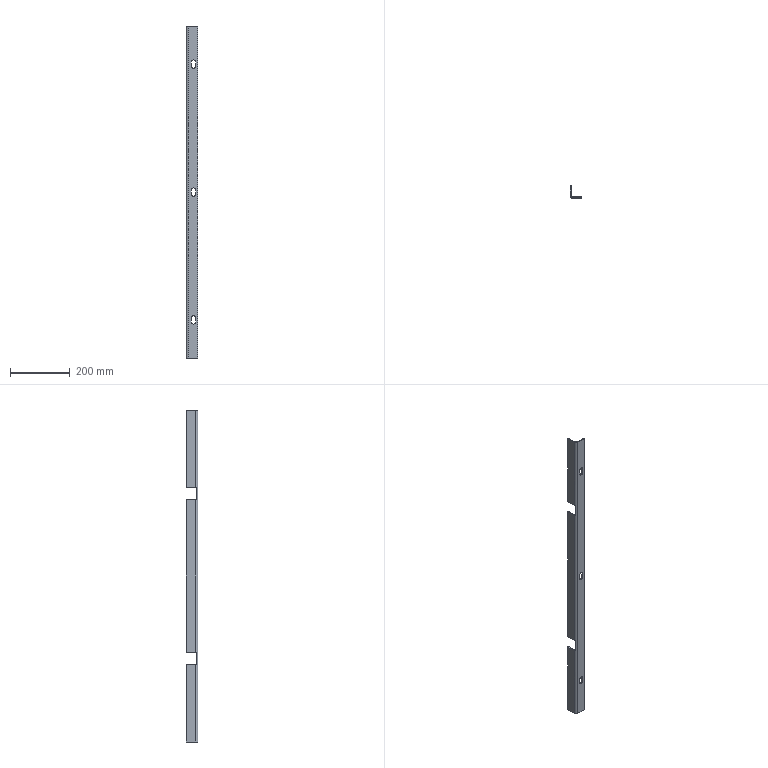Part | SolidWorks | features ICE 2, LPattern 2, ExtruThin 1, RefAxis 1 | 1 solid | 37 faces | box 40 x 40 x 1116 mm | volume 311301 mm3 | plane 24 | cylinder 13 | commonest cylinder face diameters 14 x9 8 x3 16 x1
STEP:
#1=CARTESIAN_POINT('',(25.,0.,1002.));
#2=VERTEX_POINT('',#1);
#3=CARTESIAN_POINT('',(32.,0.,995.));
#4=VERTEX_POINT('',#3);
#5=CARTESIAN_POINT('',(25.,0.,995.));
#6=DIRECTION('',(0.,1.,0.));
#7=DIRECTION('',(0.,0.,1.));
#8=AXIS2_PLACEMENT_3D('',#5,#6,#7);
#9=CIRCLE('',#8,7.);
#10=EDGE_CURVE('',#2,#4,#9,.T.);
#11=ORIENTED_EDGE('',*,*,#10,.F.);
#12=CARTESIAN_POINT('',(25.,4.,1002.));
#13=VERTEX_POINT('',#12);
#14=CARTESIAN_POINT('',(25.,-6.,1002.));
#15=DIRECTION('',(0.,1.,0.));
#16=VECTOR('',#15,1000.);
#17=LINE('',#14,#16);
#18=EDGE_CURVE('',#2,#13,#17,.T.);
#19=ORIENTED_EDGE('',*,*,#18,.T.);
#20=CARTESIAN_POINT('',(32.,4.,995.));
#21=VERTEX_POINT('',#20);
#22=CARTESIAN_POINT('',(25.,4.,995.));
#23=DIRECTION('',(0.,1.,0.));
#24=DIRECTION('',(0.,0.,1.));
#25=AXIS2_PLACEMENT_3D('',#22,#23,#24);
#26=CIRCLE('',#25,7.);
#27=EDGE_CURVE('',#13,#21,#26,.T.);
#28=ORIENTED_EDGE('',*,*,#27,.T.);
#29=CARTESIAN_POINT('',(32.,-6.,995.));
#30=DIRECTION('',(0.,1.,0.));
#31=VECTOR('',#30,1000.);
#32=LINE('',#29,#31);
#33=EDGE_CURVE('',#4,#21,#32,.T.);
#34=ORIENTED_EDGE('',*,*,#33,.F.);
#35=EDGE_LOOP('',(#11,#19,#28,#34));
#36=FACE_OUTER_BOUND('',#35,.T.);
#37=CARTESIAN_POINT('',(25.,-6.,995.));
#38=DIRECTION('',(0.,1.,0.));
#39=DIRECTION('',(0.,0.,1.));
#40=AXIS2_PLACEMENT_3D('',#37,#38,#39);
#41=CYLINDRICAL_SURFACE('',#40,7.);
#42=ADVANCED_FACE('',(#36),#41,.F.);
#43=CARTESIAN_POINT('',(25.,0.,142.));
#44=VERTEX_POINT('',#43);
#45=CARTESIAN_POINT('',(32.,0.,135.));
#46=VERTEX_POINT('',#45);
#47=CARTESIAN_POINT('',(25.,0.,135.));
#48=DIRECTION('',(0.,1.,0.));
#49=DIRECTION('',(0.,0.,1.));
#50=AXIS2_PLACEMENT_3D('',#47,#48,#49);
#51=CIRCLE('',#50,7.);
#52=EDGE_CURVE('',#44,#46,#51,.T.);
#53=ORIENTED_EDGE('',*,*,#52,.F.);
#54=CARTESIAN_POINT('',(25.,4.,142.));
#55=VERTEX_POINT('',#54);
#56=CARTESIAN_POINT('',(25.,-6.,142.));
#57=DIRECTION('',(0.,1.,0.));
#58=VECTOR('',#57,1000.);
#59=LINE('',#56,#58);
#60=EDGE_CURVE('',#44,#55,#59,.T.);
#61=ORIENTED_EDGE('',*,*,#60,.T.);
#62=CARTESIAN_POINT('',(32.,4.,135.));
#63=VERTEX_POINT('',#62);
#64=CARTESIAN_POINT('',(25.,4.,135.));
#65=DIRECTION('',(0.,1.,0.));
#66=DIRECTION('',(0.,0.,1.));
#67=AXIS2_PLACEMENT_3D('',#64,#65,#66);
#68=CIRCLE('',#67,7.);
#69=EDGE_CURVE('',#55,#63,#68,.T.);
#70=ORIENTED_EDGE('',*,*,#69,.T.);
#71=CARTESIAN_POINT('',(32.,-6.,135.));
#72=DIRECTION('',(0.,1.,0.));
#73=VECTOR('',#72,1000.);
#74=LINE('',#71,#73);
#75=EDGE_CURVE('',#46,#63,#74,.T.);
#76=ORIENTED_EDGE('',*,*,#75,.F.);
#77=EDGE_LOOP('',(#53,#61,#70,#76));
#78=FACE_OUTER_BOUND('',#77,.T.);
#79=CARTESIAN_POINT('',(25.,-6.,135.));
#80=DIRECTION('',(0.,1.,0.));
#81=DIRECTION('',(0.,0.,1.));
#82=AXIS2_PLACEMENT_3D('',#79,#80,#81);
#83=CYLINDRICAL_SURFACE('',#82,7.);
#84=ADVANCED_FACE('',(#78),#83,.F.);
#85=CARTESIAN_POINT('',(25.,0.,572.));
#86=VERTEX_POINT('',#85);
#87=CARTESIAN_POINT('',(32.,0.,565.));
#88=VERTEX_POINT('',#87);
#89=CARTESIAN_POINT('',(25.,0.,565.));
#90=DIRECTION('',(0.,1.,0.));
#91=DIRECTION('',(0.,0.,1.));
#92=AXIS2_PLACEMENT_3D('',#89,#90,#91);
#93=CIRCLE('',#92,7.);
#94=EDGE_CURVE('',#86,#88,#93,.T.);
#95=ORIENTED_EDGE('',*,*,#94,.F.);
#96=CARTESIAN_POINT('',(25.,4.,572.));
#97=VERTEX_POINT('',#96);
#98=CARTESIAN_POINT('',(25.,-6.,572.));
#99=DIRECTION('',(0.,1.,0.));
#100=VECTOR('',#99,1000.);
#101=LINE('',#98,#100);
#102=EDGE_CURVE('',#86,#97,#101,.T.);
#103=ORIENTED_EDGE('',*,*,#102,.T.);
#104=CARTESIAN_POINT('',(32.,4.,565.));
#105=VERTEX_POINT('',#104);
#106=CARTESIAN_POINT('',(25.,4.,565.));
#107=DIRECTION('',(0.,1.,0.));
#108=DIRECTION('',(0.,0.,1.));
#109=AXIS2_PLACEMENT_3D('',#106,#107,#108);
#110=CIRCLE('',#109,7.);
#111=EDGE_CURVE('',#97,#105,#110,.T.);
#112=ORIENTED_EDGE('',*,*,#111,.T.);
#113=CARTESIAN_POINT('',(32.,-6.,565.));
#114=DIRECTION('',(0.,1.,0.));
#115=VECTOR('',#114,1000.);
#116=LINE('',#113,#115);
#117=EDGE_CURVE('',#88,#105,#116,.T.);
#118=ORIENTED_EDGE('',*,*,#117,.F.);
#119=EDGE_LOOP('',(#95,#103,#112,#118));
#120=FACE_OUTER_BOUND('',#119,.T.);
#121=CARTESIAN_POINT('',(25.,-6.,565.));
#122=DIRECTION('',(0.,1.,0.));
#123=DIRECTION('',(0.,0.,1.));
#124=AXIS2_PLACEMENT_3D('',#121,#122,#123);
#125=CYLINDRICAL_SURFACE('',#124,7.);
#126=ADVANCED_FACE('',(#120),#125,.F.);
#127=CARTESIAN_POINT('',(4.,8.,857.));
#128=VERTEX_POINT('',#127);
#129=CARTESIAN_POINT('',(8.,4.,857.));
#130=VERTEX_POINT('',#129);
#131=CARTESIAN_POINT('',(8.,8.,857.));
#132=DIRECTION('',(0.,0.,1.));
#133=DIRECTION('',(1.,0.,0.));
#134=AXIS2_PLACEMENT_3D('',#131,#132,#133);
#135=CIRCLE('',#134,4.);
#136=EDGE_CURVE('',#128,#130,#135,.T.);
#137=ORIENTED_EDGE('',*,*,#136,.F.);
#138=CARTESIAN_POINT('',(4.,8.,1116.));
#139=VERTEX_POINT('',#138);
#140=CARTESIAN_POINT('',(4.,8.,1116.));
#141=DIRECTION('',(0.,0.,-1.));
#142=VECTOR('',#141,1000.);
#143=LINE('',#140,#142);
#144=EDGE_CURVE('',#139,#128,#143,.T.);
#145=ORIENTED_EDGE('',*,*,#144,.F.);
#146=CARTESIAN_POINT('',(8.,4.,1116.));
#147=VERTEX_POINT('',#146);
#148=CARTESIAN_POINT('',(8.,8.,1116.));
#149=DIRECTION('',(0.,0.,1.));
#150=DIRECTION('',(1.,0.,0.));
#151=AXIS2_PLACEMENT_3D('',#148,#149,#150);
#152=CIRCLE('',#151,4.);
#153=EDGE_CURVE('',#139,#147,#152,.T.);
#154=ORIENTED_EDGE('',*,*,#153,.T.);
#155=CARTESIAN_POINT('',(8.,4.,1116.));
#156=DIRECTION('',(0.,0.,-1.));
#157=VECTOR('',#156,1000.);
#158=LINE('',#155,#157);
#159=EDGE_CURVE('',#147,#130,#158,.T.);
#160=ORIENTED_EDGE('',*,*,#159,.T.);
#161=EDGE_LOOP('',(#137,#145,#154,#160));
#162=FACE_OUTER_BOUND('',#161,.T.);
#163=CARTESIAN_POINT('',(8.,8.,1116.));
#164=DIRECTION('',(0.,0.,-1.));
#165=DIRECTION('',(-1.,0.,0.));
#166=AXIS2_PLACEMENT_3D('',#163,#164,#165);
#167=CYLINDRICAL_SURFACE('',#166,4.);
#168=ADVANCED_FACE('',(#162),#167,.F.);
#169=CARTESIAN_POINT('',(4.,40.,857.));
#170=VERTEX_POINT('',#169);
#171=CARTESIAN_POINT('',(4.,8.,857.));
#172=DIRECTION('',(0.,-1.,0.));
#173=VECTOR('',#172,1000.);
#174=LINE('',#171,#173);
#175=EDGE_CURVE('',#170,#128,#174,.T.);
#176=ORIENTED_EDGE('',*,*,#175,.F.);
#177=CARTESIAN_POINT('',(4.,40.,1116.));
#178=VERTEX_POINT('',#177);
#179=CARTESIAN_POINT('',(4.,40.,1116.));
#180=DIRECTION('',(0.,0.,-1.));
#181=VECTOR('',#180,1000.);
#182=LINE('',#179,#181);
#183=EDGE_CURVE('',#178,#170,#182,.T.);
#184=ORIENTED_EDGE('',*,*,#183,.F.);
#185=CARTESIAN_POINT('',(4.,8.,1116.));
#186=DIRECTION('',(0.,-1.,0.));
#187=VECTOR('',#186,1000.);
#188=LINE('',#185,#187);
#189=EDGE_CURVE('',#178,#139,#188,.T.);
#190=ORIENTED_EDGE('',*,*,#189,.T.);
#191=ORIENTED_EDGE('',*,*,#144,.T.);
#192=EDGE_LOOP('',(#176,#184,#190,#191));
#193=FACE_OUTER_BOUND('',#192,.T.);
#194=CARTESIAN_POINT('',(4.,8.,1116.));
#195=DIRECTION('',(1.,0.,0.));
#196=DIRECTION('',(0.,1.,0.));
#197=AXIS2_PLACEMENT_3D('',#194,#195,#196);
#198=PLANE('',#197);
#199=ADVANCED_FACE('',(#193),#198,.T.);
#200=CARTESIAN_POINT('',(0.,40.,857.));
#201=VERTEX_POINT('',#200);
#202=CARTESIAN_POINT('',(0.,40.,857.));
#203=DIRECTION('',(1.,0.,0.));
#204=VECTOR('',#203,1000.);
#205=LINE('',#202,#204);
#206=EDGE_CURVE('',#201,#170,#205,.T.);
#207=ORIENTED_EDGE('',*,*,#206,.F.);
#208=CARTESIAN_POINT('',(0.,40.,1116.));
#209=VERTEX_POINT('',#208);
#210=CARTESIAN_POINT('',(0.,40.,1116.));
#211=DIRECTION('',(0.,0.,-1.));
#212=VECTOR('',#211,1000.);
#213=LINE('',#210,#212);
#214=EDGE_CURVE('',#209,#201,#213,.T.);
#215=ORIENTED_EDGE('',*,*,#214,.F.);
#216=CARTESIAN_POINT('',(0.,40.,1116.));
#217=DIRECTION('',(1.,0.,0.));
#218=VECTOR('',#217,1000.);
#219=LINE('',#216,#218);
#220=EDGE_CURVE('',#209,#178,#219,.T.);
#221=ORIENTED_EDGE('',*,*,#220,.T.);
#222=ORIENTED_EDGE('',*,*,#183,.T.);
#223=EDGE_LOOP('',(#207,#215,#221,#222));
#224=FACE_OUTER_BOUND('',#223,.T.);
#225=CARTESIAN_POINT('',(0.,40.,1116.));
#226=DIRECTION('',(0.,1.,0.));
#227=DIRECTION('',(-1.,0.,0.));
#228=AXIS2_PLACEMENT_3D('',#225,#226,#227);
#229=PLANE('',#228);
#230=ADVANCED_FACE('',(#224),#229,.T.);
#231=ORIENTED_EDGE('',*,*,#214,.T.);
#232=CARTESIAN_POINT('',(0.,8.,857.));
#233=VERTEX_POINT('',#232);
#234=CARTESIAN_POINT('',(0.,54.,857.));
#235=DIRECTION('',(0.,-1.,0.));
#236=VECTOR('',#235,1000.);
#237=LINE('',#234,#236);
#238=EDGE_CURVE('',#201,#233,#237,.T.);
#239=ORIENTED_EDGE('',*,*,#238,.T.);
#240=CARTESIAN_POINT('',(0.,8.,1116.));
#241=VERTEX_POINT('',#240);
#242=CARTESIAN_POINT('',(0.,8.,1116.));
#243=DIRECTION('',(0.,0.,-1.));
#244=VECTOR('',#243,1000.);
#245=LINE('',#242,#244);
#246=EDGE_CURVE('',#241,#233,#245,.T.);
#247=ORIENTED_EDGE('',*,*,#246,.F.);
#248=CARTESIAN_POINT('',(0.,8.,1116.));
#249=DIRECTION('',(0.,-1.,0.));
#250=VECTOR('',#249,1000.);
#251=LINE('',#248,#250);
#252=EDGE_CURVE('',#209,#241,#251,.T.);
#253=ORIENTED_EDGE('',*,*,#252,.F.);
#254=EDGE_LOOP('',(#231,#239,#247,#253));
#255=FACE_OUTER_BOUND('',#254,.T.);
#256=CARTESIAN_POINT('',(0.,8.,1116.));
#257=DIRECTION('',(1.,0.,0.));
#258=DIRECTION('',(0.,1.,0.));
#259=AXIS2_PLACEMENT_3D('',#256,#257,#258);
#260=PLANE('',#259);
#261=ADVANCED_FACE('',(#255),#260,.F.);
#262=CARTESIAN_POINT('',(8.,4.,815.));
#263=VERTEX_POINT('',#262);
#264=CARTESIAN_POINT('',(4.,8.,815.));
#265=VERTEX_POINT('',#264);
#266=CARTESIAN_POINT('',(8.,8.,815.));
#267=DIRECTION('',(0.,0.,-1.));
#268=DIRECTION('',(-1.,0.,0.));
#269=AXIS2_PLACEMENT_3D('',#266,#267,#268);
#270=CIRCLE('',#269,4.);
#271=EDGE_CURVE('',#263,#265,#270,.T.);
#272=ORIENTED_EDGE('',*,*,#271,.F.);
#273=CARTESIAN_POINT('',(8.,4.,301.));
#274=VERTEX_POINT('',#273);
#275=CARTESIAN_POINT('',(8.,4.,1116.));
#276=DIRECTION('',(0.,0.,-1.));
#277=VECTOR('',#276,1000.);
#278=LINE('',#275,#277);
#279=EDGE_CURVE('',#263,#274,#278,.T.);
#280=ORIENTED_EDGE('',*,*,#279,.T.);
#281=CARTESIAN_POINT('',(4.,8.,301.));
#282=VERTEX_POINT('',#281);
#283=CARTESIAN_POINT('',(8.,8.,301.));
#284=DIRECTION('',(0.,0.,1.));
#285=DIRECTION('',(1.,0.,0.));
#286=AXIS2_PLACEMENT_3D('',#283,#284,#285);
#287=CIRCLE('',#286,4.);
#288=EDGE_CURVE('',#282,#274,#287,.T.);
#289=ORIENTED_EDGE('',*,*,#288,.F.);
#290=CARTESIAN_POINT('',(4.,8.,1116.));
#291=DIRECTION('',(0.,0.,-1.));
#292=VECTOR('',#291,1000.);
#293=LINE('',#290,#292);
#294=EDGE_CURVE('',#265,#282,#293,.T.);
#295=ORIENTED_EDGE('',*,*,#294,.F.);
#296=EDGE_LOOP('',(#272,#280,#289,#295));
#297=FACE_OUTER_BOUND('',#296,.T.);
#298=CARTESIAN_POINT('',(8.,8.,1116.));
#299=DIRECTION('',(0.,0.,-1.));
#300=DIRECTION('',(-1.,0.,0.));
#301=AXIS2_PLACEMENT_3D('',#298,#299,#300);
#302=CYLINDRICAL_SURFACE('',#301,4.);
#303=ADVANCED_FACE('',(#297),#302,.F.);
#304=CARTESIAN_POINT('',(4.,40.,815.));
#305=VERTEX_POINT('',#304);
#306=CARTESIAN_POINT('',(4.,8.,815.));
#307=DIRECTION('',(0.,1.,0.));
#308=VECTOR('',#307,1000.);
#309=LINE('',#306,#308);
#310=EDGE_CURVE('',#265,#305,#309,.T.);
#311=ORIENTED_EDGE('',*,*,#310,.F.);
#312=ORIENTED_EDGE('',*,*,#294,.T.);
#313=CARTESIAN_POINT('',(4.,40.,301.));
#314=VERTEX_POINT('',#313);
#315=CARTESIAN_POINT('',(4.,8.,301.));
#316=DIRECTION('',(0.,-1.,0.));
#317=VECTOR('',#316,1000.);
#318=LINE('',#315,#317);
#319=EDGE_CURVE('',#314,#282,#318,.T.);
#320=ORIENTED_EDGE('',*,*,#319,.F.);
#321=CARTESIAN_POINT('',(4.,40.,1116.));
#322=DIRECTION('',(0.,0.,-1.));
#323=VECTOR('',#322,1000.);
#324=LINE('',#321,#323);
#325=EDGE_CURVE('',#305,#314,#324,.T.);
#326=ORIENTED_EDGE('',*,*,#325,.F.);
#327=EDGE_LOOP('',(#311,#312,#320,#326));
#328=FACE_OUTER_BOUND('',#327,.T.);
#329=CARTESIAN_POINT('',(4.,8.,1116.));
#330=DIRECTION('',(1.,0.,0.));
#331=DIRECTION('',(0.,1.,0.));
#332=AXIS2_PLACEMENT_3D('',#329,#330,#331);
#333=PLANE('',#332);
#334=ADVANCED_FACE('',(#328),#333,.T.);
#335=CARTESIAN_POINT('',(0.,40.,815.));
#336=VERTEX_POINT('',#335);
#337=CARTESIAN_POINT('',(0.,40.,815.));
#338=DIRECTION('',(-1.,0.,0.));
#339=VECTOR('',#338,1000.);
#340=LINE('',#337,#339);
#341=EDGE_CURVE('',#305,#336,#340,.T.);
#342=ORIENTED_EDGE('',*,*,#341,.F.);
#343=ORIENTED_EDGE('',*,*,#325,.T.);
#344=CARTESIAN_POINT('',(0.,40.,301.));
#345=VERTEX_POINT('',#344);
#346=CARTESIAN_POINT('',(0.,40.,301.));
#347=DIRECTION('',(1.,0.,0.));
#348=VECTOR('',#347,1000.);
#349=LINE('',#346,#348);
#350=EDGE_CURVE('',#345,#314,#349,.T.);
#351=ORIENTED_EDGE('',*,*,#350,.F.);
#352=CARTESIAN_POINT('',(0.,40.,1116.));
#353=DIRECTION('',(0.,0.,-1.));
#354=VECTOR('',#353,1000.);
#355=LINE('',#352,#354);
#356=EDGE_CURVE('',#336,#345,#355,.T.);
#357=ORIENTED_EDGE('',*,*,#356,.F.);
#358=EDGE_LOOP('',(#342,#343,#351,#357));
#359=FACE_OUTER_BOUND('',#358,.T.);
#360=CARTESIAN_POINT('',(0.,40.,1116.));
#361=DIRECTION('',(0.,1.,0.));
#362=DIRECTION('',(-1.,0.,0.));
#363=AXIS2_PLACEMENT_3D('',#360,#361,#362);
#364=PLANE('',#363);
#365=ADVANCED_FACE('',(#359),#364,.T.);
#366=CARTESIAN_POINT('',(0.,8.,815.));
#367=VERTEX_POINT('',#366);
#368=CARTESIAN_POINT('',(0.,8.,301.));
#369=VERTEX_POINT('',#368);
#370=CARTESIAN_POINT('',(0.,8.,1116.));
#371=DIRECTION('',(0.,0.,-1.));
#372=VECTOR('',#371,1000.);
#373=LINE('',#370,#372);
#374=EDGE_CURVE('',#367,#369,#373,.T.);
#375=ORIENTED_EDGE('',*,*,#374,.F.);
#376=CARTESIAN_POINT('',(0.,54.,815.));
#377=DIRECTION('',(0.,1.,0.));
#378=VECTOR('',#377,1000.);
#379=LINE('',#376,#378);
#380=EDGE_CURVE('',#367,#336,#379,.T.);
#381=ORIENTED_EDGE('',*,*,#380,.T.);
#382=ORIENTED_EDGE('',*,*,#356,.T.);
#383=CARTESIAN_POINT('',(0.,54.,301.));
#384=DIRECTION('',(0.,-1.,0.));
#385=VECTOR('',#384,1000.);
#386=LINE('',#383,#385);
#387=EDGE_CURVE('',#345,#369,#386,.T.);
#388=ORIENTED_EDGE('',*,*,#387,.T.);
#389=EDGE_LOOP('',(#375,#381,#382,#388));
#390=FACE_OUTER_BOUND('',#389,.T.);
#391=CARTESIAN_POINT('',(0.,8.,1116.));
#392=DIRECTION('',(1.,0.,0.));
#393=DIRECTION('',(0.,1.,0.));
#394=AXIS2_PLACEMENT_3D('',#391,#392,#393);
#395=PLANE('',#394);
#396=ADVANCED_FACE('',(#390),#395,.F.);
#397=CARTESIAN_POINT('',(32.,0.,981.));
#398=VERTEX_POINT('',#397);
#399=CARTESIAN_POINT('',(32.,0.,1116.));
#400=DIRECTION('',(0.,0.,-1.));
#401=VECTOR('',#400,1000.);
#402=LINE('',#399,#401);
#403=EDGE_CURVE('',#4,#398,#402,.T.);
#404=ORIENTED_EDGE('',*,*,#403,.T.);
#405=CARTESIAN_POINT('',(18.,0.,981.));
#406=VERTEX_POINT('',#405);
#407=CARTESIAN_POINT('',(25.,0.,981.));
#408=DIRECTION('',(0.,1.,0.));
#409=DIRECTION('',(0.,0.,1.));
#410=AXIS2_PLACEMENT_3D('',#407,#408,#409);
#411=CIRCLE('',#410,7.);
#412=EDGE_CURVE('',#398,#406,#411,.T.);
#413=ORIENTED_EDGE('',*,*,#412,.T.);
#414=CARTESIAN_POINT('',(18.,0.,995.));
#415=VERTEX_POINT('',#414);
#416=CARTESIAN_POINT('',(18.,0.,1116.));
#417=DIRECTION('',(0.,0.,1.));
#418=VECTOR('',#417,1000.);
#419=LINE('',#416,#418);
#420=EDGE_CURVE('',#406,#415,#419,.T.);
#421=ORIENTED_EDGE('',*,*,#420,.T.);
#422=CARTESIAN_POINT('',(25.,0.,995.));
#423=DIRECTION('',(0.,1.,0.));
#424=DIRECTION('',(0.,0.,1.));
#425=AXIS2_PLACEMENT_3D('',#422,#423,#424);
#426=CIRCLE('',#425,7.);
#427=EDGE_CURVE('',#415,#2,#426,.T.);
#428=ORIENTED_EDGE('',*,*,#427,.T.);
#429=ORIENTED_EDGE('',*,*,#10,.T.);
#430=EDGE_LOOP('',(#404,#413,#421,#428,#429));
#431=FACE_BOUND('',#430,.T.);
#432=CARTESIAN_POINT('',(32.,0.,121.));
#433=VERTEX_POINT('',#432);
#434=CARTESIAN_POINT('',(32.,0.,1116.));
#435=DIRECTION('',(0.,0.,-1.));
#436=VECTOR('',#435,1000.);
#437=LINE('',#434,#436);
#438=EDGE_CURVE('',#46,#433,#437,.T.);
#439=ORIENTED_EDGE('',*,*,#438,.T.);
#440=CARTESIAN_POINT('',(18.,0.,121.));
#441=VERTEX_POINT('',#440);
#442=CARTESIAN_POINT('',(25.,0.,121.));
#443=DIRECTION('',(0.,1.,0.));
#444=DIRECTION('',(0.,0.,1.));
#445=AXIS2_PLACEMENT_3D('',#442,#443,#444);
#446=CIRCLE('',#445,7.);
#447=EDGE_CURVE('',#433,#441,#446,.T.);
#448=ORIENTED_EDGE('',*,*,#447,.T.);
#449=CARTESIAN_POINT('',(18.,0.,135.));
#450=VERTEX_POINT('',#449);
#451=CARTESIAN_POINT('',(18.,0.,1116.));
#452=DIRECTION('',(0.,0.,1.));
#453=VECTOR('',#452,1000.);
#454=LINE('',#451,#453);
#455=EDGE_CURVE('',#441,#450,#454,.T.);
#456=ORIENTED_EDGE('',*,*,#455,.T.);
#457=CARTESIAN_POINT('',(25.,0.,135.));
#458=DIRECTION('',(0.,1.,0.));
#459=DIRECTION('',(0.,0.,1.));
#460=AXIS2_PLACEMENT_3D('',#457,#458,#459);
#461=CIRCLE('',#460,7.);
#462=EDGE_CURVE('',#450,#44,#461,.T.);
#463=ORIENTED_EDGE('',*,*,#462,.T.);
#464=ORIENTED_EDGE('',*,*,#52,.T.);
#465=EDGE_LOOP('',(#439,#448,#456,#463,#464));
#466=FACE_BOUND('',#465,.T.);
#467=CARTESIAN_POINT('',(32.,0.,551.));
#468=VERTEX_POINT('',#467);
#469=CARTESIAN_POINT('',(32.,0.,1116.));
#470=DIRECTION('',(0.,0.,-1.));
#471=VECTOR('',#470,1000.);
#472=LINE('',#469,#471);
#473=EDGE_CURVE('',#88,#468,#472,.T.);
#474=ORIENTED_EDGE('',*,*,#473,.T.);
#475=CARTESIAN_POINT('',(18.,0.,551.));
#476=VERTEX_POINT('',#475);
#477=CARTESIAN_POINT('',(25.,0.,551.));
#478=DIRECTION('',(0.,1.,0.));
#479=DIRECTION('',(0.,0.,1.));
#480=AXIS2_PLACEMENT_3D('',#477,#478,#479);
#481=CIRCLE('',#480,7.);
#482=EDGE_CURVE('',#468,#476,#481,.T.);
#483=ORIENTED_EDGE('',*,*,#482,.T.);
#484=CARTESIAN_POINT('',(18.,0.,565.));
#485=VERTEX_POINT('',#484);
#486=CARTESIAN_POINT('',(18.,0.,1116.));
#487=DIRECTION('',(0.,0.,1.));
#488=VECTOR('',#487,1000.);
#489=LINE('',#486,#488);
#490=EDGE_CURVE('',#476,#485,#489,.T.);
#491=ORIENTED_EDGE('',*,*,#490,.T.);
#492=CARTESIAN_POINT('',(25.,0.,565.));
#493=DIRECTION('',(0.,1.,0.));
#494=DIRECTION('',(0.,0.,1.));
#495=AXIS2_PLACEMENT_3D('',#492,#493,#494);
#496=CIRCLE('',#495,7.);
#497=EDGE_CURVE('',#485,#86,#496,.T.);
#498=ORIENTED_EDGE('',*,*,#497,.T.);
#499=ORIENTED_EDGE('',*,*,#94,.T.);
#500=EDGE_LOOP('',(#474,#483,#491,#498,#499));
#501=FACE_BOUND('',#500,.T.);
#502=CARTESIAN_POINT('',(8.,0.,0.));
#503=VERTEX_POINT('',#502);
#504=CARTESIAN_POINT('',(40.,0.,0.));
#505=VERTEX_POINT('',#504);
#506=CARTESIAN_POINT('',(8.,0.,0.));
#507=DIRECTION('',(1.,0.,0.));
#508=VECTOR('',#507,1000.);
#509=LINE('',#506,#508);
#510=EDGE_CURVE('',#503,#505,#509,.T.);
#511=ORIENTED_EDGE('',*,*,#510,.T.);
#512=CARTESIAN_POINT('',(40.,0.,1116.));
#513=VERTEX_POINT('',#512);
#514=CARTESIAN_POINT('',(40.,0.,1116.));
#515=DIRECTION('',(0.,0.,-1.));
#516=VECTOR('',#515,1000.);
#517=LINE('',#514,#516);
#518=EDGE_CURVE('',#513,#505,#517,.T.);
#519=ORIENTED_EDGE('',*,*,#518,.F.);
#520=CARTESIAN_POINT('',(8.,0.,1116.));
#521=VERTEX_POINT('',#520);
#522=CARTESIAN_POINT('',(8.,0.,1116.));
#523=DIRECTION('',(1.,0.,0.));
#524=VECTOR('',#523,1000.);
#525=LINE('',#522,#524);
#526=EDGE_CURVE('',#521,#513,#525,.T.);
#527=ORIENTED_EDGE('',*,*,#526,.F.);
#528=CARTESIAN_POINT('',(8.,0.,1116.));
#529=DIRECTION('',(0.,0.,-1.));
#530=VECTOR('',#529,1000.);
#531=LINE('',#528,#530);
#532=EDGE_CURVE('',#521,#503,#531,.T.);
#533=ORIENTED_EDGE('',*,*,#532,.T.);
#534=EDGE_LOOP('',(#511,#519,#527,#533));
#535=FACE_OUTER_BOUND('',#534,.T.);
#536=CARTESIAN_POINT('',(8.,0.,1116.));
#537=DIRECTION('',(0.,1.,0.));
#538=DIRECTION('',(0.,0.,1.));
#539=AXIS2_PLACEMENT_3D('',#536,#537,#538);
#540=PLANE('',#539);
#541=ADVANCED_FACE('',(#431,#466,#501,#535),#540,.F.);
#542=CARTESIAN_POINT('',(40.,4.,0.));
#543=VERTEX_POINT('',#542);
#544=CARTESIAN_POINT('',(40.,4.,0.));
#545=DIRECTION('',(0.,-1.,0.));
#546=VECTOR('',#545,1000.);
#547=LINE('',#544,#546);
#548=EDGE_CURVE('',#543,#505,#547,.T.);
#549=ORIENTED_EDGE('',*,*,#548,.F.);
#550=CARTESIAN_POINT('',(40.,4.,1116.));
#551=VERTEX_POINT('',#550);
#552=CARTESIAN_POINT('',(40.,4.,1116.));
#553=DIRECTION('',(0.,0.,-1.));
#554=VECTOR('',#553,1000.);
#555=LINE('',#552,#554);
#556=EDGE_CURVE('',#551,#543,#555,.T.);
#557=ORIENTED_EDGE('',*,*,#556,.F.);
#558=CARTESIAN_POINT('',(40.,4.,1116.));
#559=DIRECTION('',(0.,-1.,0.));
#560=VECTOR('',#559,1000.);
#561=LINE('',#558,#560);
#562=EDGE_CURVE('',#551,#513,#561,.T.);
#563=ORIENTED_EDGE('',*,*,#562,.T.);
#564=ORIENTED_EDGE('',*,*,#518,.T.);
#565=EDGE_LOOP('',(#549,#557,#563,#564));
#566=FACE_OUTER_BOUND('',#565,.T.);
#567=CARTESIAN_POINT('',(40.,4.,1116.));
#568=DIRECTION('',(1.,0.,0.));
#569=DIRECTION('',(0.,0.,-1.));
#570=AXIS2_PLACEMENT_3D('',#567,#568,#569);
#571=PLANE('',#570);
#572=ADVANCED_FACE('',(#566),#571,.T.);
#573=CARTESIAN_POINT('',(32.,4.,981.));
#574=VERTEX_POINT('',#573);
#575=CARTESIAN_POINT('',(18.,4.,981.));
#576=VERTEX_POINT('',#575);
#577=CARTESIAN_POINT('',(25.,4.,981.));
#578=DIRECTION('',(0.,1.,0.));
#579=DIRECTION('',(0.,0.,1.));
#580=AXIS2_PLACEMENT_3D('',#577,#578,#579);
#581=CIRCLE('',#580,7.);
#582=EDGE_CURVE('',#574,#576,#581,.T.);
#583=ORIENTED_EDGE('',*,*,#582,.F.);
#584=CARTESIAN_POINT('',(32.,4.,981.));
#585=DIRECTION('',(0.,0.,-1.));
#586=VECTOR('',#585,1000.);
#587=LINE('',#584,#586);
#588=EDGE_CURVE('',#21,#574,#587,.T.);
#589=ORIENTED_EDGE('',*,*,#588,.F.);
#590=ORIENTED_EDGE('',*,*,#27,.F.);
#591=CARTESIAN_POINT('',(18.,4.,995.));
#592=VERTEX_POINT('',#591);
#593=CARTESIAN_POINT('',(25.,4.,995.));
#594=DIRECTION('',(0.,1.,0.));
#595=DIRECTION('',(0.,0.,1.));
#596=AXIS2_PLACEMENT_3D('',#593,#594,#595);
#597=CIRCLE('',#596,7.);
#598=EDGE_CURVE('',#592,#13,#597,.T.);
#599=ORIENTED_EDGE('',*,*,#598,.F.);
#600=CARTESIAN_POINT('',(18.,4.,981.));
#601=DIRECTION('',(0.,0.,1.));
#602=VECTOR('',#601,1000.);
#603=LINE('',#600,#602);
#604=EDGE_CURVE('',#576,#592,#603,.T.);
#605=ORIENTED_EDGE('',*,*,#604,.F.);
#606=EDGE_LOOP('',(#583,#589,#590,#599,#605));
#607=FACE_BOUND('',#606,.T.);
#608=CARTESIAN_POINT('',(32.,4.,121.));
#609=VERTEX_POINT('',#608);
#610=CARTESIAN_POINT('',(18.,4.,121.));
#611=VERTEX_POINT('',#610);
#612=CARTESIAN_POINT('',(25.,4.,121.));
#613=DIRECTION('',(0.,1.,0.));
#614=DIRECTION('',(0.,0.,1.));
#615=AXIS2_PLACEMENT_3D('',#612,#613,#614);
#616=CIRCLE('',#615,7.);
#617=EDGE_CURVE('',#609,#611,#616,.T.);
#618=ORIENTED_EDGE('',*,*,#617,.F.);
#619=CARTESIAN_POINT('',(32.,4.,121.));
#620=DIRECTION('',(0.,0.,-1.));
#621=VECTOR('',#620,1000.);
#622=LINE('',#619,#621);
#623=EDGE_CURVE('',#63,#609,#622,.T.);
#624=ORIENTED_EDGE('',*,*,#623,.F.);
#625=ORIENTED_EDGE('',*,*,#69,.F.);
#626=CARTESIAN_POINT('',(18.,4.,135.));
#627=VERTEX_POINT('',#626);
#628=CARTESIAN_POINT('',(25.,4.,135.));
#629=DIRECTION('',(0.,1.,0.));
#630=DIRECTION('',(0.,0.,1.));
#631=AXIS2_PLACEMENT_3D('',#628,#629,#630);
#632=CIRCLE('',#631,7.);
#633=EDGE_CURVE('',#627,#55,#632,.T.);
#634=ORIENTED_EDGE('',*,*,#633,.F.);
#635=CARTESIAN_POINT('',(18.,4.,121.));
#636=DIRECTION('',(0.,0.,1.));
#637=VECTOR('',#636,1000.);
#638=LINE('',#635,#637);
#639=EDGE_CURVE('',#611,#627,#638,.T.);
#640=ORIENTED_EDGE('',*,*,#639,.F.);
#641=EDGE_LOOP('',(#618,#624,#625,#634,#640));
#642=FACE_BOUND('',#641,.T.);
#643=CARTESIAN_POINT('',(32.,4.,551.));
#644=VERTEX_POINT('',#643);
#645=CARTESIAN_POINT('',(18.,4.,551.));
#646=VERTEX_POINT('',#645);
#647=CARTESIAN_POINT('',(25.,4.,551.));
#648=DIRECTION('',(0.,1.,0.));
#649=DIRECTION('',(0.,0.,1.));
#650=AXIS2_PLACEMENT_3D('',#647,#648,#649);
#651=CIRCLE('',#650,7.);
#652=EDGE_CURVE('',#644,#646,#651,.T.);
#653=ORIENTED_EDGE('',*,*,#652,.F.);
#654=CARTESIAN_POINT('',(32.,4.,551.));
#655=DIRECTION('',(0.,0.,-1.));
#656=VECTOR('',#655,1000.);
#657=LINE('',#654,#656);
#658=EDGE_CURVE('',#105,#644,#657,.T.);
#659=ORIENTED_EDGE('',*,*,#658,.F.);
#660=ORIENTED_EDGE('',*,*,#111,.F.);
#661=CARTESIAN_POINT('',(18.,4.,565.));
#662=VERTEX_POINT('',#661);
#663=CARTESIAN_POINT('',(25.,4.,565.));
#664=DIRECTION('',(0.,1.,0.));
#665=DIRECTION('',(0.,0.,1.));
#666=AXIS2_PLACEMENT_3D('',#663,#664,#665);
#667=CIRCLE('',#666,7.);
#668=EDGE_CURVE('',#662,#97,#667,.T.);
#669=ORIENTED_EDGE('',*,*,#668,.F.);
#670=CARTESIAN_POINT('',(18.,4.,551.));
#671=DIRECTION('',(0.,0.,1.));
#672=VECTOR('',#671,1000.);
#673=LINE('',#670,#672);
#674=EDGE_CURVE('',#646,#662,#673,.T.);
#675=ORIENTED_EDGE('',*,*,#674,.F.);
#676=EDGE_LOOP('',(#653,#659,#660,#669,#675));
#677=FACE_BOUND('',#676,.T.);
#678=ORIENTED_EDGE('',*,*,#279,.F.);
#679=CARTESIAN_POINT('',(1.072,4.,815.));
#680=VERTEX_POINT('',#679);
#681=CARTESIAN_POINT('',(0.,4.,815.));
#682=DIRECTION('',(1.,0.,0.));
#683=VECTOR('',#682,1000.);
#684=LINE('',#681,#683);
#685=EDGE_CURVE('',#680,#263,#684,.T.);
#686=ORIENTED_EDGE('',*,*,#685,.F.);
#687=CARTESIAN_POINT('',(1.072,4.,857.));
#688=VERTEX_POINT('',#687);
#689=CARTESIAN_POINT('',(1.072,4.,1116.));
#690=DIRECTION('',(0.,0.,-1.));
#691=VECTOR('',#690,1000.);
#692=LINE('',#689,#691);
#693=EDGE_CURVE('',#688,#680,#692,.T.);
#694=ORIENTED_EDGE('',*,*,#693,.F.);
#695=CARTESIAN_POINT('',(0.,4.,857.));
#696=DIRECTION('',(1.,0.,0.));
#697=VECTOR('',#696,1000.);
#698=LINE('',#695,#697);
#699=EDGE_CURVE('',#688,#130,#698,.T.);
#700=ORIENTED_EDGE('',*,*,#699,.T.);
#701=ORIENTED_EDGE('',*,*,#159,.F.);
#702=CARTESIAN_POINT('',(8.,4.,1116.));
#703=DIRECTION('',(1.,0.,0.));
#704=VECTOR('',#703,1000.);
#705=LINE('',#702,#704);
#706=EDGE_CURVE('',#147,#551,#705,.T.);
#707=ORIENTED_EDGE('',*,*,#706,.T.);
#708=ORIENTED_EDGE('',*,*,#556,.T.);
#709=CARTESIAN_POINT('',(8.,4.,0.));
#710=VERTEX_POINT('',#709);
#711=CARTESIAN_POINT('',(8.,4.,0.));
#712=DIRECTION('',(1.,0.,0.));
#713=VECTOR('',#712,1000.);
#714=LINE('',#711,#713);
#715=EDGE_CURVE('',#710,#543,#714,.T.);
#716=ORIENTED_EDGE('',*,*,#715,.F.);
#717=CARTESIAN_POINT('',(8.,4.,259.));
#718=VERTEX_POINT('',#717);
#719=CARTESIAN_POINT('',(8.,4.,1116.));
#720=DIRECTION('',(0.,0.,-1.));
#721=VECTOR('',#720,1000.);
#722=LINE('',#719,#721);
#723=EDGE_CURVE('',#718,#710,#722,.T.);
#724=ORIENTED_EDGE('',*,*,#723,.F.);
#725=CARTESIAN_POINT('',(1.072,4.,259.));
#726=VERTEX_POINT('',#725);
#727=CARTESIAN_POINT('',(0.,4.,259.));
#728=DIRECTION('',(1.,0.,0.));
#729=VECTOR('',#728,1000.);
#730=LINE('',#727,#729);
#731=EDGE_CURVE('',#726,#718,#730,.T.);
#732=ORIENTED_EDGE('',*,*,#731,.F.);
#733=CARTESIAN_POINT('',(1.072,4.,301.));
#734=VERTEX_POINT('',#733);
#735=CARTESIAN_POINT('',(1.072,4.,1116.));
#736=DIRECTION('',(0.,0.,-1.));
#737=VECTOR('',#736,1000.);
#738=LINE('',#735,#737);
#739=EDGE_CURVE('',#734,#726,#738,.T.);
#740=ORIENTED_EDGE('',*,*,#739,.F.);
#741=CARTESIAN_POINT('',(0.,4.,301.));
#742=DIRECTION('',(1.,0.,0.));
#743=VECTOR('',#742,1000.);
#744=LINE('',#741,#743);
#745=EDGE_CURVE('',#734,#274,#744,.T.);
#746=ORIENTED_EDGE('',*,*,#745,.T.);
#747=EDGE_LOOP('',(#678,#686,#694,#700,#701,#707,#708,#716,#724,#732,#740,#746));
#748=FACE_OUTER_BOUND('',#747,.T.);
#749=CARTESIAN_POINT('',(8.,4.,1116.));
#750=DIRECTION('',(0.,1.,0.));
#751=DIRECTION('',(0.,0.,1.));
#752=AXIS2_PLACEMENT_3D('',#749,#750,#751);
#753=PLANE('',#752);
#754=ADVANCED_FACE('',(#607,#642,#677,#748),#753,.T.);
#755=CARTESIAN_POINT('',(4.,8.,259.));
#756=VERTEX_POINT('',#755);
#757=CARTESIAN_POINT('',(8.,8.,259.));
#758=DIRECTION('',(0.,0.,-1.));
#759=DIRECTION('',(-1.,0.,0.));
#760=AXIS2_PLACEMENT_3D('',#757,#758,#759);
#761=CIRCLE('',#760,4.);
#762=EDGE_CURVE('',#718,#756,#761,.T.);
#763=ORIENTED_EDGE('',*,*,#762,.F.);
#764=ORIENTED_EDGE('',*,*,#723,.T.);
#765=CARTESIAN_POINT('',(4.,8.,0.));
#766=VERTEX_POINT('',#765);
#767=CARTESIAN_POINT('',(8.,8.,0.));
#768=DIRECTION('',(0.,0.,1.));
#769=DIRECTION('',(1.,0.,0.));
#770=AXIS2_PLACEMENT_3D('',#767,#768,#769);
#771=CIRCLE('',#770,4.);
#772=EDGE_CURVE('',#766,#710,#771,.T.);
#773=ORIENTED_EDGE('',*,*,#772,.F.);
#774=CARTESIAN_POINT('',(4.,8.,1116.));
#775=DIRECTION('',(0.,0.,-1.));
#776=VECTOR('',#775,1000.);
#777=LINE('',#774,#776);
#778=EDGE_CURVE('',#756,#766,#777,.T.);
#779=ORIENTED_EDGE('',*,*,#778,.F.);
#780=EDGE_LOOP('',(#763,#764,#773,#779));
#781=FACE_OUTER_BOUND('',#780,.T.);
#782=CARTESIAN_POINT('',(8.,8.,1116.));
#783=DIRECTION('',(0.,0.,-1.));
#784=DIRECTION('',(-1.,0.,0.));
#785=AXIS2_PLACEMENT_3D('',#782,#783,#784);
#786=CYLINDRICAL_SURFACE('',#785,4.);
#787=ADVANCED_FACE('',(#781),#786,.F.);
#788=CARTESIAN_POINT('',(4.,40.,259.));
#789=VERTEX_POINT('',#788);
#790=CARTESIAN_POINT('',(4.,8.,259.));
#791=DIRECTION('',(0.,1.,0.));
#792=VECTOR('',#791,1000.);
#793=LINE('',#790,#792);
#794=EDGE_CURVE('',#756,#789,#793,.T.);
#795=ORIENTED_EDGE('',*,*,#794,.F.);
#796=ORIENTED_EDGE('',*,*,#778,.T.);
#797=CARTESIAN_POINT('',(4.,40.,0.));
#798=VERTEX_POINT('',#797);
#799=CARTESIAN_POINT('',(4.,8.,0.));
#800=DIRECTION('',(0.,-1.,0.));
#801=VECTOR('',#800,1000.);
#802=LINE('',#799,#801);
#803=EDGE_CURVE('',#798,#766,#802,.T.);
#804=ORIENTED_EDGE('',*,*,#803,.F.);
#805=CARTESIAN_POINT('',(4.,40.,1116.));
#806=DIRECTION('',(0.,0.,-1.));
#807=VECTOR('',#806,1000.);
#808=LINE('',#805,#807);
#809=EDGE_CURVE('',#789,#798,#808,.T.);
#810=ORIENTED_EDGE('',*,*,#809,.F.);
#811=EDGE_LOOP('',(#795,#796,#804,#810));
#812=FACE_OUTER_BOUND('',#811,.T.);
#813=CARTESIAN_POINT('',(4.,8.,1116.));
#814=DIRECTION('',(1.,0.,0.));
#815=DIRECTION('',(0.,1.,0.));
#816=AXIS2_PLACEMENT_3D('',#813,#814,#815);
#817=PLANE('',#816);
#818=ADVANCED_FACE('',(#812),#817,.T.);
#819=CARTESIAN_POINT('',(0.,40.,259.));
#820=VERTEX_POINT('',#819);
#821=CARTESIAN_POINT('',(0.,40.,259.));
#822=DIRECTION('',(-1.,0.,0.));
#823=VECTOR('',#822,1000.);
#824=LINE('',#821,#823);
#825=EDGE_CURVE('',#789,#820,#824,.T.);
#826=ORIENTED_EDGE('',*,*,#825,.F.);
#827=ORIENTED_EDGE('',*,*,#809,.T.);
#828=CARTESIAN_POINT('',(0.,40.,0.));
#829=VERTEX_POINT('',#828);
#830=CARTESIAN_POINT('',(0.,40.,0.));
#831=DIRECTION('',(1.,0.,0.));
#832=VECTOR('',#831,1000.);
#833=LINE('',#830,#832);
#834=EDGE_CURVE('',#829,#798,#833,.T.);
#835=ORIENTED_EDGE('',*,*,#834,.F.);
#836=CARTESIAN_POINT('',(0.,40.,1116.));
#837=DIRECTION('',(0.,0.,-1.));
#838=VECTOR('',#837,1000.);
#839=LINE('',#836,#838);
#840=EDGE_CURVE('',#820,#829,#839,.T.);
#841=ORIENTED_EDGE('',*,*,#840,.F.);
#842=EDGE_LOOP('',(#826,#827,#835,#841));
#843=FACE_OUTER_BOUND('',#842,.T.);
#844=CARTESIAN_POINT('',(0.,40.,1116.));
#845=DIRECTION('',(0.,1.,0.));
#846=DIRECTION('',(-1.,0.,0.));
#847=AXIS2_PLACEMENT_3D('',#844,#845,#846);
#848=PLANE('',#847);
#849=ADVANCED_FACE('',(#843),#848,.T.);
#850=CARTESIAN_POINT('',(0.,8.,259.));
#851=VERTEX_POINT('',#850);
#852=CARTESIAN_POINT('',(0.,8.,0.));
#853=VERTEX_POINT('',#852);
#854=CARTESIAN_POINT('',(0.,8.,1116.));
#855=DIRECTION('',(0.,0.,-1.));
#856=VECTOR('',#855,1000.);
#857=LINE('',#854,#856);
#858=EDGE_CURVE('',#851,#853,#857,.T.);
#859=ORIENTED_EDGE('',*,*,#858,.F.);
#860=CARTESIAN_POINT('',(0.,54.,259.));
#861=DIRECTION('',(0.,1.,0.));
#862=VECTOR('',#861,1000.);
#863=LINE('',#860,#862);
#864=EDGE_CURVE('',#851,#820,#863,.T.);
#865=ORIENTED_EDGE('',*,*,#864,.T.);
#866=ORIENTED_EDGE('',*,*,#840,.T.);
#867=CARTESIAN_POINT('',(0.,8.,0.));
#868=DIRECTION('',(0.,-1.,0.));
#869=VECTOR('',#868,1000.);
#870=LINE('',#867,#869);
#871=EDGE_CURVE('',#829,#853,#870,.T.);
#872=ORIENTED_EDGE('',*,*,#871,.T.);
#873=EDGE_LOOP('',(#859,#865,#866,#872));
#874=FACE_OUTER_BOUND('',#873,.T.);
#875=CARTESIAN_POINT('',(0.,8.,1116.));
#876=DIRECTION('',(1.,0.,0.));
#877=DIRECTION('',(0.,1.,0.));
#878=AXIS2_PLACEMENT_3D('',#875,#876,#877);
#879=PLANE('',#878);
#880=ADVANCED_FACE('',(#874),#879,.F.);
#881=ORIENTED_EDGE('',*,*,#246,.T.);
#882=CARTESIAN_POINT('',(8.,8.,857.));
#883=DIRECTION('',(0.,0.,1.));
#884=DIRECTION('',(1.,0.,0.));
#885=AXIS2_PLACEMENT_3D('',#882,#883,#884);
#886=CIRCLE('',#885,8.);
#887=EDGE_CURVE('',#233,#688,#886,.T.);
#888=ORIENTED_EDGE('',*,*,#887,.T.);
#889=ORIENTED_EDGE('',*,*,#693,.T.);
#890=CARTESIAN_POINT('',(8.,8.,815.));
#891=DIRECTION('',(0.,0.,-1.));
#892=DIRECTION('',(-1.,0.,0.));
#893=AXIS2_PLACEMENT_3D('',#890,#891,#892);
#894=CIRCLE('',#893,8.);
#895=EDGE_CURVE('',#680,#367,#894,.T.);
#896=ORIENTED_EDGE('',*,*,#895,.T.);
#897=ORIENTED_EDGE('',*,*,#374,.T.);
#898=CARTESIAN_POINT('',(8.,8.,301.));
#899=DIRECTION('',(0.,0.,1.));
#900=DIRECTION('',(1.,0.,0.));
#901=AXIS2_PLACEMENT_3D('',#898,#899,#900);
#902=CIRCLE('',#901,8.);
#903=EDGE_CURVE('',#369,#734,#902,.T.);
#904=ORIENTED_EDGE('',*,*,#903,.T.);
#905=ORIENTED_EDGE('',*,*,#739,.T.);
#906=CARTESIAN_POINT('',(8.,8.,259.));
#907=DIRECTION('',(0.,0.,-1.));
#908=DIRECTION('',(-1.,0.,0.));
#909=AXIS2_PLACEMENT_3D('',#906,#907,#908);
#910=CIRCLE('',#909,8.);
#911=EDGE_CURVE('',#726,#851,#910,.T.);
#912=ORIENTED_EDGE('',*,*,#911,.T.);
#913=ORIENTED_EDGE('',*,*,#858,.T.);
#914=CARTESIAN_POINT('',(8.,8.,0.));
#915=DIRECTION('',(0.,0.,1.));
#916=DIRECTION('',(1.,0.,0.));
#917=AXIS2_PLACEMENT_3D('',#914,#915,#916);
#918=CIRCLE('',#917,8.);
#919=EDGE_CURVE('',#853,#503,#918,.T.);
#920=ORIENTED_EDGE('',*,*,#919,.T.);
#921=ORIENTED_EDGE('',*,*,#532,.F.);
#922=CARTESIAN_POINT('',(8.,8.,1116.));
#923=DIRECTION('',(0.,0.,1.));
#924=DIRECTION('',(1.,0.,0.));
#925=AXIS2_PLACEMENT_3D('',#922,#923,#924);
#926=CIRCLE('',#925,8.);
#927=EDGE_CURVE('',#241,#521,#926,.T.);
#928=ORIENTED_EDGE('',*,*,#927,.F.);
#929=EDGE_LOOP('',(#881,#888,#889,#896,#897,#904,#905,#912,#913,#920,#921,#928));
#930=FACE_OUTER_BOUND('',#929,.T.);
#931=CARTESIAN_POINT('',(8.,8.,1116.));
#932=DIRECTION('',(0.,0.,-1.));
#933=DIRECTION('',(-1.,0.,0.));
#934=AXIS2_PLACEMENT_3D('',#931,#932,#933);
#935=CYLINDRICAL_SURFACE('',#934,8.);
#936=ADVANCED_FACE('',(#930),#935,.T.);
#937=ORIENTED_EDGE('',*,*,#526,.T.);
#938=ORIENTED_EDGE('',*,*,#562,.F.);
#939=ORIENTED_EDGE('',*,*,#706,.F.);
#940=ORIENTED_EDGE('',*,*,#153,.F.);
#941=ORIENTED_EDGE('',*,*,#189,.F.);
#942=ORIENTED_EDGE('',*,*,#220,.F.);
#943=ORIENTED_EDGE('',*,*,#252,.T.);
#944=ORIENTED_EDGE('',*,*,#927,.T.);
#945=EDGE_LOOP('',(#937,#938,#939,#940,#941,#942,#943,#944));
#946=FACE_OUTER_BOUND('',#945,.T.);
#947=CARTESIAN_POINT('',(8.,8.,1116.));
#948=DIRECTION('',(0.,0.,1.));
#949=DIRECTION('',(1.,0.,0.));
#950=AXIS2_PLACEMENT_3D('',#947,#948,#949);
#951=PLANE('',#950);
#952=ADVANCED_FACE('',(#946),#951,.T.);
#953=ORIENTED_EDGE('',*,*,#510,.F.);
#954=ORIENTED_EDGE('',*,*,#919,.F.);
#955=ORIENTED_EDGE('',*,*,#871,.F.);
#956=ORIENTED_EDGE('',*,*,#834,.T.);
#957=ORIENTED_EDGE('',*,*,#803,.T.);
#958=ORIENTED_EDGE('',*,*,#772,.T.);
#959=ORIENTED_EDGE('',*,*,#715,.T.);
#960=ORIENTED_EDGE('',*,*,#548,.T.);
#961=EDGE_LOOP('',(#953,#954,#955,#956,#957,#958,#959,#960));
#962=FACE_OUTER_BOUND('',#961,.T.);
#963=CARTESIAN_POINT('',(8.,8.,0.));
#964=DIRECTION('',(0.,0.,1.));
#965=DIRECTION('',(1.,0.,0.));
#966=AXIS2_PLACEMENT_3D('',#963,#964,#965);
#967=PLANE('',#966);
#968=ADVANCED_FACE('',(#962),#967,.F.);
#969=ORIENTED_EDGE('',*,*,#288,.T.);
#970=ORIENTED_EDGE('',*,*,#745,.F.);
#971=ORIENTED_EDGE('',*,*,#903,.F.);
#972=ORIENTED_EDGE('',*,*,#387,.F.);
#973=ORIENTED_EDGE('',*,*,#350,.T.);
#974=ORIENTED_EDGE('',*,*,#319,.T.);
#975=EDGE_LOOP('',(#969,#970,#971,#972,#973,#974));
#976=FACE_OUTER_BOUND('',#975,.T.);
#977=CARTESIAN_POINT('',(0.,54.,301.));
#978=DIRECTION('',(0.,0.,1.));
#979=DIRECTION('',(1.,0.,0.));
#980=AXIS2_PLACEMENT_3D('',#977,#978,#979);
#981=PLANE('',#980);
#982=ADVANCED_FACE('',(#976),#981,.F.);
#983=ORIENTED_EDGE('',*,*,#762,.T.);
#984=ORIENTED_EDGE('',*,*,#794,.T.);
#985=ORIENTED_EDGE('',*,*,#825,.T.);
#986=ORIENTED_EDGE('',*,*,#864,.F.);
#987=ORIENTED_EDGE('',*,*,#911,.F.);
#988=ORIENTED_EDGE('',*,*,#731,.T.);
#989=EDGE_LOOP('',(#983,#984,#985,#986,#987,#988));
#990=FACE_OUTER_BOUND('',#989,.T.);
#991=CARTESIAN_POINT('',(0.,54.,259.));
#992=DIRECTION('',(0.,0.,-1.));
#993=DIRECTION('',(-1.,0.,0.));
#994=AXIS2_PLACEMENT_3D('',#991,#992,#993);
#995=PLANE('',#994);
#996=ADVANCED_FACE('',(#990),#995,.F.);
#997=ORIENTED_EDGE('',*,*,#136,.T.);
#998=ORIENTED_EDGE('',*,*,#699,.F.);
#999=ORIENTED_EDGE('',*,*,#887,.F.);
#1000=ORIENTED_EDGE('',*,*,#238,.F.);
#1001=ORIENTED_EDGE('',*,*,#206,.T.);
#1002=ORIENTED_EDGE('',*,*,#175,.T.);
#1003=EDGE_LOOP('',(#997,#998,#999,#1000,#1001,#1002));
#1004=FACE_OUTER_BOUND('',#1003,.T.);
#1005=CARTESIAN_POINT('',(0.,54.,857.));
#1006=DIRECTION('',(0.,0.,1.));
#1007=DIRECTION('',(1.,0.,0.));
#1008=AXIS2_PLACEMENT_3D('',#1005,#1006,#1007);
#1009=PLANE('',#1008);
#1010=ADVANCED_FACE('',(#1004),#1009,.F.);
#1011=ORIENTED_EDGE('',*,*,#271,.T.);
#1012=ORIENTED_EDGE('',*,*,#310,.T.);
#1013=ORIENTED_EDGE('',*,*,#341,.T.);
#1014=ORIENTED_EDGE('',*,*,#380,.F.);
#1015=ORIENTED_EDGE('',*,*,#895,.F.);
#1016=ORIENTED_EDGE('',*,*,#685,.T.);
#1017=EDGE_LOOP('',(#1011,#1012,#1013,#1014,#1015,#1016));
#1018=FACE_OUTER_BOUND('',#1017,.T.);
#1019=CARTESIAN_POINT('',(0.,54.,815.));
#1020=DIRECTION('',(0.,0.,-1.));
#1021=DIRECTION('',(-1.,0.,0.));
#1022=AXIS2_PLACEMENT_3D('',#1019,#1020,#1021);
#1023=PLANE('',#1022);
#1024=ADVANCED_FACE('',(#1018),#1023,.F.);
#1025=CARTESIAN_POINT('',(32.,-6.,551.));
#1026=DIRECTION('',(0.,1.,0.));
#1027=VECTOR('',#1026,1000.);
#1028=LINE('',#1025,#1027);
#1029=EDGE_CURVE('',#468,#644,#1028,.T.);
#1030=ORIENTED_EDGE('',*,*,#1029,.T.);
#1031=ORIENTED_EDGE('',*,*,#652,.T.);
#1032=CARTESIAN_POINT('',(18.,-6.,551.));
#1033=DIRECTION('',(0.,1.,0.));
#1034=VECTOR('',#1033,1000.);
#1035=LINE('',#1032,#1034);
#1036=EDGE_CURVE('',#476,#646,#1035,.T.);
#1037=ORIENTED_EDGE('',*,*,#1036,.F.);
#1038=ORIENTED_EDGE('',*,*,#482,.F.);
#1039=EDGE_LOOP('',(#1030,#1031,#1037,#1038));
#1040=FACE_OUTER_BOUND('',#1039,.T.);
#1041=CARTESIAN_POINT('',(25.,-6.,551.));
#1042=DIRECTION('',(0.,1.,0.));
#1043=DIRECTION('',(0.,0.,1.));
#1044=AXIS2_PLACEMENT_3D('',#1041,#1042,#1043);
#1045=CYLINDRICAL_SURFACE('',#1044,7.);
#1046=ADVANCED_FACE('',(#1040),#1045,.F.);
#1047=ORIENTED_EDGE('',*,*,#117,.T.);
#1048=ORIENTED_EDGE('',*,*,#658,.T.);
#1049=ORIENTED_EDGE('',*,*,#1029,.F.);
#1050=ORIENTED_EDGE('',*,*,#473,.F.);
#1051=EDGE_LOOP('',(#1047,#1048,#1049,#1050));
#1052=FACE_OUTER_BOUND('',#1051,.T.);
#1053=CARTESIAN_POINT('',(32.,-6.,551.));
#1054=DIRECTION('',(1.,0.,0.));
#1055=DIRECTION('',(0.,0.,-1.));
#1056=AXIS2_PLACEMENT_3D('',#1053,#1054,#1055);
#1057=PLANE('',#1056);
#1058=ADVANCED_FACE('',(#1052),#1057,.F.);
#1059=ORIENTED_EDGE('',*,*,#102,.F.);
#1060=ORIENTED_EDGE('',*,*,#497,.F.);
#1061=CARTESIAN_POINT('',(18.,-6.,565.));
#1062=DIRECTION('',(0.,1.,0.));
#1063=VECTOR('',#1062,1000.);
#1064=LINE('',#1061,#1063);
#1065=EDGE_CURVE('',#485,#662,#1064,.T.);
#1066=ORIENTED_EDGE('',*,*,#1065,.T.);
#1067=ORIENTED_EDGE('',*,*,#668,.T.);
#1068=EDGE_LOOP('',(#1059,#1060,#1066,#1067));
#1069=FACE_OUTER_BOUND('',#1068,.T.);
#1070=CARTESIAN_POINT('',(25.,-6.,565.));
#1071=DIRECTION('',(0.,1.,0.));
#1072=DIRECTION('',(0.,0.,1.));
#1073=AXIS2_PLACEMENT_3D('',#1070,#1071,#1072);
#1074=CYLINDRICAL_SURFACE('',#1073,7.);
#1075=ADVANCED_FACE('',(#1069),#1074,.F.);
#1076=ORIENTED_EDGE('',*,*,#1036,.T.);
#1077=ORIENTED_EDGE('',*,*,#674,.T.);
#1078=ORIENTED_EDGE('',*,*,#1065,.F.);
#1079=ORIENTED_EDGE('',*,*,#490,.F.);
#1080=EDGE_LOOP('',(#1076,#1077,#1078,#1079));
#1081=FACE_OUTER_BOUND('',#1080,.T.);
#1082=CARTESIAN_POINT('',(18.,-6.,551.));
#1083=DIRECTION('',(-1.,0.,0.));
#1084=DIRECTION('',(0.,0.,1.));
#1085=AXIS2_PLACEMENT_3D('',#1082,#1083,#1084);
#1086=PLANE('',#1085);
#1087=ADVANCED_FACE('',(#1081),#1086,.F.);
#1088=CARTESIAN_POINT('',(32.,-6.,121.));
#1089=DIRECTION('',(0.,1.,0.));
#1090=VECTOR('',#1089,1000.);
#1091=LINE('',#1088,#1090);
#1092=EDGE_CURVE('',#433,#609,#1091,.T.);
#1093=ORIENTED_EDGE('',*,*,#1092,.T.);
#1094=ORIENTED_EDGE('',*,*,#617,.T.);
#1095=CARTESIAN_POINT('',(18.,-6.,121.));
#1096=DIRECTION('',(0.,1.,0.));
#1097=VECTOR('',#1096,1000.);
#1098=LINE('',#1095,#1097);
#1099=EDGE_CURVE('',#441,#611,#1098,.T.);
#1100=ORIENTED_EDGE('',*,*,#1099,.F.);
#1101=ORIENTED_EDGE('',*,*,#447,.F.);
#1102=EDGE_LOOP('',(#1093,#1094,#1100,#1101));
#1103=FACE_OUTER_BOUND('',#1102,.T.);
#1104=CARTESIAN_POINT('',(25.,-6.,121.));
#1105=DIRECTION('',(0.,1.,0.));
#1106=DIRECTION('',(0.,0.,1.));
#1107=AXIS2_PLACEMENT_3D('',#1104,#1105,#1106);
#1108=CYLINDRICAL_SURFACE('',#1107,7.);
#1109=ADVANCED_FACE('',(#1103),#1108,.F.);
#1110=ORIENTED_EDGE('',*,*,#75,.T.);
#1111=ORIENTED_EDGE('',*,*,#623,.T.);
#1112=ORIENTED_EDGE('',*,*,#1092,.F.);
#1113=ORIENTED_EDGE('',*,*,#438,.F.);
#1114=EDGE_LOOP('',(#1110,#1111,#1112,#1113));
#1115=FACE_OUTER_BOUND('',#1114,.T.);
#1116=CARTESIAN_POINT('',(32.,-6.,121.));
#1117=DIRECTION('',(1.,0.,0.));
#1118=DIRECTION('',(0.,0.,-1.));
#1119=AXIS2_PLACEMENT_3D('',#1116,#1117,#1118);
#1120=PLANE('',#1119);
#1121=ADVANCED_FACE('',(#1115),#1120,.F.);
#1122=ORIENTED_EDGE('',*,*,#60,.F.);
#1123=ORIENTED_EDGE('',*,*,#462,.F.);
#1124=CARTESIAN_POINT('',(18.,-6.,135.));
#1125=DIRECTION('',(0.,1.,0.));
#1126=VECTOR('',#1125,1000.);
#1127=LINE('',#1124,#1126);
#1128=EDGE_CURVE('',#450,#627,#1127,.T.);
#1129=ORIENTED_EDGE('',*,*,#1128,.T.);
#1130=ORIENTED_EDGE('',*,*,#633,.T.);
#1131=EDGE_LOOP('',(#1122,#1123,#1129,#1130));
#1132=FACE_OUTER_BOUND('',#1131,.T.);
#1133=CARTESIAN_POINT('',(25.,-6.,135.));
#1134=DIRECTION('',(0.,1.,0.));
#1135=DIRECTION('',(0.,0.,1.));
#1136=AXIS2_PLACEMENT_3D('',#1133,#1134,#1135);
#1137=CYLINDRICAL_SURFACE('',#1136,7.);
#1138=ADVANCED_FACE('',(#1132),#1137,.F.);
#1139=ORIENTED_EDGE('',*,*,#1099,.T.);
#1140=ORIENTED_EDGE('',*,*,#639,.T.);
#1141=ORIENTED_EDGE('',*,*,#1128,.F.);
#1142=ORIENTED_EDGE('',*,*,#455,.F.);
#1143=EDGE_LOOP('',(#1139,#1140,#1141,#1142));
#1144=FACE_OUTER_BOUND('',#1143,.T.);
#1145=CARTESIAN_POINT('',(18.,-6.,121.));
#1146=DIRECTION('',(-1.,0.,0.));
#1147=DIRECTION('',(0.,0.,1.));
#1148=AXIS2_PLACEMENT_3D('',#1145,#1146,#1147);
#1149=PLANE('',#1148);
#1150=ADVANCED_FACE('',(#1144),#1149,.F.);
#1151=CARTESIAN_POINT('',(32.,-6.,981.));
#1152=DIRECTION('',(0.,1.,0.));
#1153=VECTOR('',#1152,1000.);
#1154=LINE('',#1151,#1153);
#1155=EDGE_CURVE('',#398,#574,#1154,.T.);
#1156=ORIENTED_EDGE('',*,*,#1155,.T.);
#1157=ORIENTED_EDGE('',*,*,#582,.T.);
#1158=CARTESIAN_POINT('',(18.,-6.,981.));
#1159=DIRECTION('',(0.,1.,0.));
#1160=VECTOR('',#1159,1000.);
#1161=LINE('',#1158,#1160);
#1162=EDGE_CURVE('',#406,#576,#1161,.T.);
#1163=ORIENTED_EDGE('',*,*,#1162,.F.);
#1164=ORIENTED_EDGE('',*,*,#412,.F.);
#1165=EDGE_LOOP('',(#1156,#1157,#1163,#1164));
#1166=FACE_OUTER_BOUND('',#1165,.T.);
#1167=CARTESIAN_POINT('',(25.,-6.,981.));
#1168=DIRECTION('',(0.,1.,0.));
#1169=DIRECTION('',(0.,0.,1.));
#1170=AXIS2_PLACEMENT_3D('',#1167,#1168,#1169);
#1171=CYLINDRICAL_SURFACE('',#1170,7.);
#1172=ADVANCED_FACE('',(#1166),#1171,.F.);
#1173=ORIENTED_EDGE('',*,*,#33,.T.);
#1174=ORIENTED_EDGE('',*,*,#588,.T.);
#1175=ORIENTED_EDGE('',*,*,#1155,.F.);
#1176=ORIENTED_EDGE('',*,*,#403,.F.);
#1177=EDGE_LOOP('',(#1173,#1174,#1175,#1176));
#1178=FACE_OUTER_BOUND('',#1177,.T.);
#1179=CARTESIAN_POINT('',(32.,-6.,981.));
#1180=DIRECTION('',(1.,0.,0.));
#1181=DIRECTION('',(0.,0.,-1.));
#1182=AXIS2_PLACEMENT_3D('',#1179,#1180,#1181);
#1183=PLANE('',#1182);
#1184=ADVANCED_FACE('',(#1178),#1183,.F.);
#1185=ORIENTED_EDGE('',*,*,#18,.F.);
#1186=ORIENTED_EDGE('',*,*,#427,.F.);
#1187=CARTESIAN_POINT('',(18.,-6.,995.));
#1188=DIRECTION('',(0.,1.,0.));
#1189=VECTOR('',#1188,1000.);
#1190=LINE('',#1187,#1189);
#1191=EDGE_CURVE('',#415,#592,#1190,.T.);
#1192=ORIENTED_EDGE('',*,*,#1191,.T.);
#1193=ORIENTED_EDGE('',*,*,#598,.T.);
#1194=EDGE_LOOP('',(#1185,#1186,#1192,#1193));
#1195=FACE_OUTER_BOUND('',#1194,.T.);
#1196=CARTESIAN_POINT('',(25.,-6.,995.));
#1197=DIRECTION('',(0.,1.,0.));
#1198=DIRECTION('',(0.,0.,1.));
#1199=AXIS2_PLACEMENT_3D('',#1196,#1197,#1198);
#1200=CYLINDRICAL_SURFACE('',#1199,7.);
#1201=ADVANCED_FACE('',(#1195),#1200,.F.);
#1202=ORIENTED_EDGE('',*,*,#1162,.T.);
#1203=ORIENTED_EDGE('',*,*,#604,.T.);
#1204=ORIENTED_EDGE('',*,*,#1191,.F.);
#1205=ORIENTED_EDGE('',*,*,#420,.F.);
#1206=EDGE_LOOP('',(#1202,#1203,#1204,#1205));
#1207=FACE_OUTER_BOUND('',#1206,.T.);
#1208=CARTESIAN_POINT('',(18.,-6.,981.));
#1209=DIRECTION('',(-1.,0.,0.));
#1210=DIRECTION('',(0.,0.,1.));
#1211=AXIS2_PLACEMENT_3D('',#1208,#1209,#1210);
#1212=PLANE('',#1211);
#1213=ADVANCED_FACE('',(#1207),#1212,.F.);
#1214=CLOSED_SHELL('',(#42,#84,#126,#168,#199,#230,#261,#303,#334,#365,#396,#541,#572,#754,#787,#818,#849,#880,#936,#952,#968,#982,#996,#1010,#1024,#1046,#1058,#1075,#1087,#1109,#1121,#1138,#1150,#1172,#1184,#1201,#1213));
#1215=MANIFOLD_SOLID_BREP('',#1214);
#1216=CARTESIAN_POINT('',(0.,0.,0.));
#1217=DIRECTION('',(0.,0.,1.));
#1218=DIRECTION('',(1.,0.,0.));
#1219=AXIS2_PLACEMENT_3D('',#1216,#1217,#1218);
#1220=(LENGTH_UNIT()NAMED_UNIT(*)SI_UNIT(.MILLI.,.METRE.));
#1221=UNCERTAINTY_MEASURE_WITH_UNIT(LENGTH_MEASURE(0.00001),#1220,'','');
#1222=(NAMED_UNIT(*)PLANE_ANGLE_UNIT()SI_UNIT($,.RADIAN.));
#1223=(NAMED_UNIT(*)SI_UNIT($,.STERADIAN.)SOLID_ANGLE_UNIT());
#1224=(GEOMETRIC_REPRESENTATION_CONTEXT(3)GLOBAL_UNCERTAINTY_ASSIGNED_CONTEXT((#1221))GLOBAL_UNIT_ASSIGNED_CONTEXT((#1220,#1222,#1223))REPRESENTATION_CONTEXT('',''));
#1225=ADVANCED_BREP_SHAPE_REPRESENTATION('',(#1215,#1219),#1224);